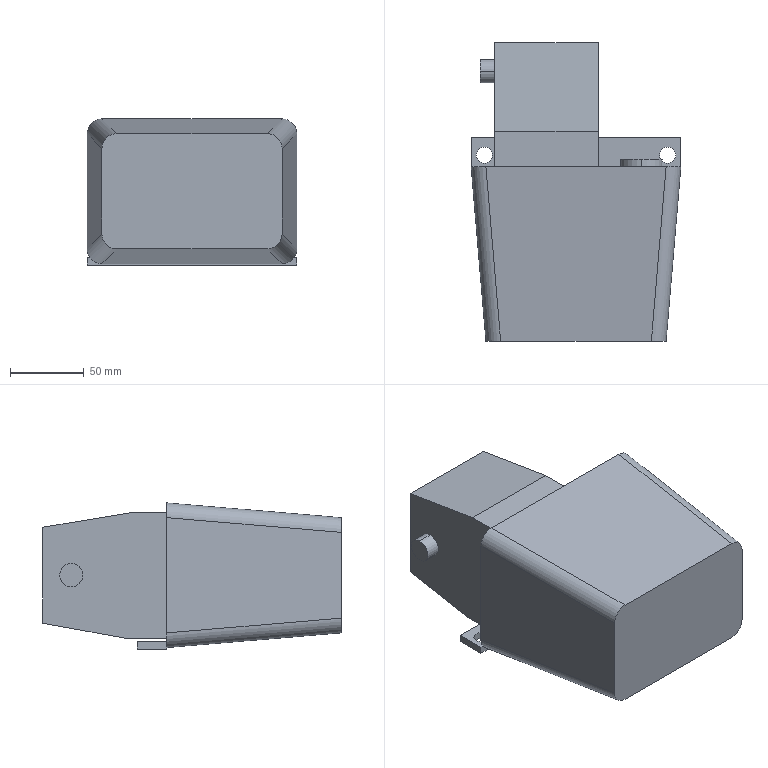Part | SolidWorks | features BaseBody 1 | 1 solid | 43 faces | box 142 x 202 x 99 mm | volume 619754 mm3 | plane 27 | cylinder 16 | commonest cylinder face diameters 11 x4 16 x4 20 x4 15.743 x2 28.298 x2
STEP:
#1=CARTESIAN_POINT('',(44.366,5.,1.458));
#2=VERTEX_POINT('',#1);
#3=CARTESIAN_POINT('',(44.366,5.,29.756));
#4=VERTEX_POINT('',#3);
#5=CARTESIAN_POINT('',(44.366,5.,15.607));
#6=DIRECTION('',(0.,-1.,0.));
#7=DIRECTION('',(0.,0.,-1.));
#8=AXIS2_PLACEMENT_3D('',#5,#6,#7);
#9=CIRCLE('',#8,14.149);
#10=EDGE_CURVE('',#2,#4,#9,.T.);
#11=ORIENTED_EDGE('',*,*,#10,.T.);
#12=CARTESIAN_POINT('',(44.366,0.,29.756));
#13=VERTEX_POINT('',#12);
#14=CARTESIAN_POINT('',(44.366,5.,29.756));
#15=DIRECTION('',(0.,-1.,0.));
#16=VECTOR('',#15,1000.);
#17=LINE('',#14,#16);
#18=EDGE_CURVE('',#4,#13,#17,.T.);
#19=ORIENTED_EDGE('',*,*,#18,.T.);
#20=CARTESIAN_POINT('',(44.366,0.,1.458));
#21=VERTEX_POINT('',#20);
#22=CARTESIAN_POINT('',(44.366,0.,15.607));
#23=DIRECTION('',(0.,-1.,0.));
#24=DIRECTION('',(0.,0.,-1.));
#25=AXIS2_PLACEMENT_3D('',#22,#23,#24);
#26=CIRCLE('',#25,14.149);
#27=EDGE_CURVE('',#21,#13,#26,.T.);
#28=ORIENTED_EDGE('',*,*,#27,.F.);
#29=CARTESIAN_POINT('',(44.366,5.,1.458));
#30=DIRECTION('',(0.,-1.,0.));
#31=VECTOR('',#30,1000.);
#32=LINE('',#29,#31);
#33=EDGE_CURVE('',#2,#21,#32,.T.);
#34=ORIENTED_EDGE('',*,*,#33,.F.);
#35=EDGE_LOOP('',(#11,#19,#28,#34));
#36=FACE_OUTER_BOUND('',#35,.T.);
#37=CARTESIAN_POINT('',(44.366,5.,15.607));
#38=DIRECTION('',(0.,-1.,0.));
#39=DIRECTION('',(0.,0.,-1.));
#40=AXIS2_PLACEMENT_3D('',#37,#38,#39);
#41=CYLINDRICAL_SURFACE('',#40,14.149);
#42=ADVANCED_FACE('',(#36),#41,.T.);
#43=CARTESIAN_POINT('',(67.5,8.,-50.));
#44=VERTEX_POINT('',#43);
#45=CARTESIAN_POINT('',(56.5,8.,-50.));
#46=VERTEX_POINT('',#45);
#47=CARTESIAN_POINT('',(62.,8.,-50.));
#48=DIRECTION('',(0.,0.,-1.));
#49=DIRECTION('',(1.,0.,0.));
#50=AXIS2_PLACEMENT_3D('',#47,#48,#49);
#51=CIRCLE('',#50,5.5);
#52=EDGE_CURVE('',#44,#46,#51,.T.);
#53=ORIENTED_EDGE('',*,*,#52,.T.);
#54=CARTESIAN_POINT('',(56.5,8.,-45.));
#55=VERTEX_POINT('',#54);
#56=CARTESIAN_POINT('',(56.5,8.,-45.));
#57=DIRECTION('',(0.,0.,1.));
#58=VECTOR('',#57,1000.);
#59=LINE('',#56,#58);
#60=EDGE_CURVE('',#46,#55,#59,.T.);
#61=ORIENTED_EDGE('',*,*,#60,.T.);
#62=CARTESIAN_POINT('',(67.5,8.,-45.));
#63=VERTEX_POINT('',#62);
#64=CARTESIAN_POINT('',(62.,8.,-45.));
#65=DIRECTION('',(0.,0.,1.));
#66=DIRECTION('',(1.,0.,0.));
#67=AXIS2_PLACEMENT_3D('',#64,#65,#66);
#68=CIRCLE('',#67,5.5);
#69=EDGE_CURVE('',#55,#63,#68,.T.);
#70=ORIENTED_EDGE('',*,*,#69,.T.);
#71=CARTESIAN_POINT('',(67.5,8.,-45.));
#72=DIRECTION('',(0.,0.,1.));
#73=VECTOR('',#72,1000.);
#74=LINE('',#71,#73);
#75=EDGE_CURVE('',#44,#63,#74,.T.);
#76=ORIENTED_EDGE('',*,*,#75,.F.);
#77=EDGE_LOOP('',(#53,#61,#70,#76));
#78=FACE_OUTER_BOUND('',#77,.T.);
#79=CARTESIAN_POINT('',(62.,8.,-45.));
#80=DIRECTION('',(0.,0.,1.));
#81=DIRECTION('',(1.,0.,0.));
#82=AXIS2_PLACEMENT_3D('',#79,#80,#81);
#83=CYLINDRICAL_SURFACE('',#82,5.5);
#84=ADVANCED_FACE('',(#78),#83,.F.);
#85=CARTESIAN_POINT('',(-56.5,8.,-50.));
#86=VERTEX_POINT('',#85);
#87=CARTESIAN_POINT('',(-67.5,8.,-50.));
#88=VERTEX_POINT('',#87);
#89=CARTESIAN_POINT('',(-62.,8.,-50.));
#90=DIRECTION('',(0.,0.,-1.));
#91=DIRECTION('',(1.,0.,0.));
#92=AXIS2_PLACEMENT_3D('',#89,#90,#91);
#93=CIRCLE('',#92,5.5);
#94=EDGE_CURVE('',#86,#88,#93,.T.);
#95=ORIENTED_EDGE('',*,*,#94,.T.);
#96=CARTESIAN_POINT('',(-67.5,8.,-45.));
#97=VERTEX_POINT('',#96);
#98=CARTESIAN_POINT('',(-67.5,8.,-45.));
#99=DIRECTION('',(0.,0.,1.));
#100=VECTOR('',#99,1000.);
#101=LINE('',#98,#100);
#102=EDGE_CURVE('',#88,#97,#101,.T.);
#103=ORIENTED_EDGE('',*,*,#102,.T.);
#104=CARTESIAN_POINT('',(-56.5,8.,-45.));
#105=VERTEX_POINT('',#104);
#106=CARTESIAN_POINT('',(-62.,8.,-45.));
#107=DIRECTION('',(0.,0.,1.));
#108=DIRECTION('',(1.,0.,0.));
#109=AXIS2_PLACEMENT_3D('',#106,#107,#108);
#110=CIRCLE('',#109,5.5);
#111=EDGE_CURVE('',#97,#105,#110,.T.);
#112=ORIENTED_EDGE('',*,*,#111,.T.);
#113=CARTESIAN_POINT('',(-56.5,8.,-45.));
#114=DIRECTION('',(0.,0.,1.));
#115=VECTOR('',#114,1000.);
#116=LINE('',#113,#115);
#117=EDGE_CURVE('',#86,#105,#116,.T.);
#118=ORIENTED_EDGE('',*,*,#117,.F.);
#119=EDGE_LOOP('',(#95,#103,#112,#118));
#120=FACE_OUTER_BOUND('',#119,.T.);
#121=CARTESIAN_POINT('',(-62.,8.,-45.));
#122=DIRECTION('',(0.,0.,1.));
#123=DIRECTION('',(1.,0.,0.));
#124=AXIS2_PLACEMENT_3D('',#121,#122,#123);
#125=CYLINDRICAL_SURFACE('',#124,5.5);
#126=ADVANCED_FACE('',(#120),#125,.F.);
#127=CARTESIAN_POINT('',(-65.,64.732,-7.871));
#128=VERTEX_POINT('',#127);
#129=CARTESIAN_POINT('',(-65.,64.732,7.871));
#130=VERTEX_POINT('',#129);
#131=CARTESIAN_POINT('',(-65.,64.732,0.));
#132=DIRECTION('',(1.,0.,0.));
#133=DIRECTION('',(0.,0.,-1.));
#134=AXIS2_PLACEMENT_3D('',#131,#132,#133);
#135=CIRCLE('',#134,7.871);
#136=EDGE_CURVE('',#128,#130,#135,.T.);
#137=ORIENTED_EDGE('',*,*,#136,.T.);
#138=CARTESIAN_POINT('',(-55.,64.732,7.871));
#139=VERTEX_POINT('',#138);
#140=CARTESIAN_POINT('',(-65.,64.732,7.871));
#141=DIRECTION('',(1.,0.,0.));
#142=VECTOR('',#141,1000.);
#143=LINE('',#140,#142);
#144=EDGE_CURVE('',#130,#139,#143,.T.);
#145=ORIENTED_EDGE('',*,*,#144,.T.);
#146=CARTESIAN_POINT('',(-55.,64.732,-7.871));
#147=VERTEX_POINT('',#146);
#148=CARTESIAN_POINT('',(-55.,64.732,0.));
#149=DIRECTION('',(-1.,0.,0.));
#150=DIRECTION('',(0.,0.,-1.));
#151=AXIS2_PLACEMENT_3D('',#148,#149,#150);
#152=CIRCLE('',#151,7.871);
#153=EDGE_CURVE('',#139,#147,#152,.T.);
#154=ORIENTED_EDGE('',*,*,#153,.T.);
#155=CARTESIAN_POINT('',(-65.,64.732,-7.871));
#156=DIRECTION('',(1.,0.,0.));
#157=VECTOR('',#156,1000.);
#158=LINE('',#155,#157);
#159=EDGE_CURVE('',#128,#147,#158,.T.);
#160=ORIENTED_EDGE('',*,*,#159,.F.);
#161=EDGE_LOOP('',(#137,#145,#154,#160));
#162=FACE_OUTER_BOUND('',#161,.T.);
#163=CARTESIAN_POINT('',(-65.,64.732,0.));
#164=DIRECTION('',(1.,0.,0.));
#165=DIRECTION('',(0.,0.,-1.));
#166=AXIS2_PLACEMENT_3D('',#163,#164,#165);
#167=CYLINDRICAL_SURFACE('',#166,7.871);
#168=ADVANCED_FACE('',(#162),#167,.T.);
#169=ORIENTED_EDGE('',*,*,#136,.F.);
#170=CARTESIAN_POINT('',(-65.,64.732,0.));
#171=DIRECTION('',(1.,0.,0.));
#172=DIRECTION('',(0.,0.,-1.));
#173=AXIS2_PLACEMENT_3D('',#170,#171,#172);
#174=CIRCLE('',#173,7.871);
#175=EDGE_CURVE('',#130,#128,#174,.T.);
#176=ORIENTED_EDGE('',*,*,#175,.F.);
#177=EDGE_LOOP('',(#169,#176));
#178=FACE_OUTER_BOUND('',#177,.T.);
#179=CARTESIAN_POINT('',(-65.,64.732,0.));
#180=DIRECTION('',(-1.,0.,0.));
#181=DIRECTION('',(0.,0.,1.));
#182=AXIS2_PLACEMENT_3D('',#179,#180,#181);
#183=PLANE('',#182);
#184=ADVANCED_FACE('',(#178),#183,.T.);
#185=ORIENTED_EDGE('',*,*,#10,.F.);
#186=CARTESIAN_POINT('',(44.366,5.,15.607));
#187=DIRECTION('',(0.,-1.,0.));
#188=DIRECTION('',(0.,0.,-1.));
#189=AXIS2_PLACEMENT_3D('',#186,#187,#188);
#190=CIRCLE('',#189,14.149);
#191=EDGE_CURVE('',#4,#2,#190,.T.);
#192=ORIENTED_EDGE('',*,*,#191,.F.);
#193=EDGE_LOOP('',(#185,#192));
#194=FACE_OUTER_BOUND('',#193,.T.);
#195=CARTESIAN_POINT('',(44.366,5.,15.607));
#196=DIRECTION('',(0.,1.,0.));
#197=DIRECTION('',(0.,0.,1.));
#198=AXIS2_PLACEMENT_3D('',#195,#196,#197);
#199=PLANE('',#198);
#200=ADVANCED_FACE('',(#194),#199,.T.);
#201=ORIENTED_EDGE('',*,*,#144,.F.);
#202=ORIENTED_EDGE('',*,*,#175,.T.);
#203=ORIENTED_EDGE('',*,*,#159,.T.);
#204=CARTESIAN_POINT('',(-55.,64.732,0.));
#205=DIRECTION('',(-1.,0.,0.));
#206=DIRECTION('',(0.,0.,-1.));
#207=AXIS2_PLACEMENT_3D('',#204,#205,#206);
#208=CIRCLE('',#207,7.871);
#209=EDGE_CURVE('',#147,#139,#208,.T.);
#210=ORIENTED_EDGE('',*,*,#209,.T.);
#211=EDGE_LOOP('',(#201,#202,#203,#210));
#212=FACE_OUTER_BOUND('',#211,.T.);
#213=CARTESIAN_POINT('',(-65.,64.732,0.));
#214=DIRECTION('',(1.,0.,0.));
#215=DIRECTION('',(0.,0.,-1.));
#216=AXIS2_PLACEMENT_3D('',#213,#214,#215);
#217=CYLINDRICAL_SURFACE('',#216,7.871);
#218=ADVANCED_FACE('',(#212),#217,.T.);
#219=CARTESIAN_POINT('',(-55.,29.,-42.5));
#220=VERTEX_POINT('',#219);
#221=CARTESIAN_POINT('',(-55.,84.,-32.5));
#222=VERTEX_POINT('',#221);
#223=CARTESIAN_POINT('',(-55.,29.,-42.5));
#224=DIRECTION('',(0.,0.9839,0.1789));
#225=VECTOR('',#224,1000.);
#226=LINE('',#223,#225);
#227=EDGE_CURVE('',#220,#222,#226,.T.);
#228=ORIENTED_EDGE('',*,*,#227,.T.);
#229=CARTESIAN_POINT('',(15.,84.,-32.5));
#230=VERTEX_POINT('',#229);
#231=CARTESIAN_POINT('',(0.,84.,-32.5));
#232=DIRECTION('',(-1.,0.,0.));
#233=VECTOR('',#232,1000.);
#234=LINE('',#231,#233);
#235=EDGE_CURVE('',#230,#222,#234,.T.);
#236=ORIENTED_EDGE('',*,*,#235,.F.);
#237=CARTESIAN_POINT('',(15.,29.,-42.5));
#238=VERTEX_POINT('',#237);
#239=CARTESIAN_POINT('',(15.,84.,-32.5));
#240=DIRECTION('',(0.,-0.9839,-0.1789));
#241=VECTOR('',#240,1000.);
#242=LINE('',#239,#241);
#243=EDGE_CURVE('',#230,#238,#242,.T.);
#244=ORIENTED_EDGE('',*,*,#243,.T.);
#245=CARTESIAN_POINT('',(-55.,29.,-42.5));
#246=DIRECTION('',(-1.,0.,0.));
#247=VECTOR('',#246,1000.);
#248=LINE('',#245,#247);
#249=EDGE_CURVE('',#238,#220,#248,.T.);
#250=ORIENTED_EDGE('',*,*,#249,.T.);
#251=EDGE_LOOP('',(#228,#236,#244,#250));
#252=FACE_OUTER_BOUND('',#251,.T.);
#253=CARTESIAN_POINT('',(71.,29.,-42.5));
#254=DIRECTION('',(0.,-0.1789,0.9839));
#255=DIRECTION('',(0.,-0.9839,-0.1789));
#256=AXIS2_PLACEMENT_3D('',#253,#254,#255);
#257=PLANE('',#256);
#258=ADVANCED_FACE('',(#252),#257,.F.);
#259=ORIENTED_EDGE('',*,*,#235,.T.);
#260=CARTESIAN_POINT('',(-55.,84.,32.5));
#261=VERTEX_POINT('',#260);
#262=CARTESIAN_POINT('',(-55.,84.,-42.5));
#263=DIRECTION('',(0.,0.,1.));
#264=VECTOR('',#263,1000.);
#265=LINE('',#262,#264);
#266=EDGE_CURVE('',#222,#261,#265,.T.);
#267=ORIENTED_EDGE('',*,*,#266,.T.);
#268=CARTESIAN_POINT('',(15.,84.,32.5));
#269=VERTEX_POINT('',#268);
#270=CARTESIAN_POINT('',(71.,84.,32.5));
#271=DIRECTION('',(1.,0.,0.));
#272=VECTOR('',#271,1000.);
#273=LINE('',#270,#272);
#274=EDGE_CURVE('',#261,#269,#273,.T.);
#275=ORIENTED_EDGE('',*,*,#274,.T.);
#276=CARTESIAN_POINT('',(15.,84.,-42.5));
#277=DIRECTION('',(0.,0.,-1.));
#278=VECTOR('',#277,1000.);
#279=LINE('',#276,#278);
#280=EDGE_CURVE('',#269,#230,#279,.T.);
#281=ORIENTED_EDGE('',*,*,#280,.T.);
#282=EDGE_LOOP('',(#259,#267,#275,#281));
#283=FACE_OUTER_BOUND('',#282,.T.);
#284=CARTESIAN_POINT('',(0.,84.,0.));
#285=DIRECTION('',(0.,1.,0.));
#286=DIRECTION('',(0.,0.,1.));
#287=AXIS2_PLACEMENT_3D('',#284,#285,#286);
#288=PLANE('',#287);
#289=ADVANCED_FACE('',(#283),#288,.T.);
#290=CARTESIAN_POINT('',(-55.,24.,42.5));
#291=VERTEX_POINT('',#290);
#292=CARTESIAN_POINT('',(-55.,84.,32.5));
#293=DIRECTION('',(0.,-0.9864,0.1644));
#294=VECTOR('',#293,1000.);
#295=LINE('',#292,#294);
#296=EDGE_CURVE('',#261,#291,#295,.T.);
#297=ORIENTED_EDGE('',*,*,#296,.T.);
#298=CARTESIAN_POINT('',(15.,24.,42.5));
#299=VERTEX_POINT('',#298);
#300=CARTESIAN_POINT('',(-55.,24.,42.5));
#301=DIRECTION('',(1.,0.,0.));
#302=VECTOR('',#301,1000.);
#303=LINE('',#300,#302);
#304=EDGE_CURVE('',#291,#299,#303,.T.);
#305=ORIENTED_EDGE('',*,*,#304,.T.);
#306=CARTESIAN_POINT('',(15.,24.,42.5));
#307=DIRECTION('',(0.,0.9864,-0.1644));
#308=VECTOR('',#307,1000.);
#309=LINE('',#306,#308);
#310=EDGE_CURVE('',#299,#269,#309,.T.);
#311=ORIENTED_EDGE('',*,*,#310,.T.);
#312=ORIENTED_EDGE('',*,*,#274,.F.);
#313=EDGE_LOOP('',(#297,#305,#311,#312));
#314=FACE_OUTER_BOUND('',#313,.T.);
#315=CARTESIAN_POINT('',(71.,84.,32.5));
#316=DIRECTION('',(0.,-0.1644,-0.9864));
#317=DIRECTION('',(0.,0.9864,-0.1644));
#318=AXIS2_PLACEMENT_3D('',#315,#316,#317);
#319=PLANE('',#318);
#320=ADVANCED_FACE('',(#314),#319,.F.);
#321=ORIENTED_EDGE('',*,*,#102,.F.);
#322=CARTESIAN_POINT('',(-62.,8.,-50.));
#323=DIRECTION('',(0.,0.,-1.));
#324=DIRECTION('',(1.,0.,0.));
#325=AXIS2_PLACEMENT_3D('',#322,#323,#324);
#326=CIRCLE('',#325,5.5);
#327=EDGE_CURVE('',#88,#86,#326,.T.);
#328=ORIENTED_EDGE('',*,*,#327,.T.);
#329=ORIENTED_EDGE('',*,*,#117,.T.);
#330=CARTESIAN_POINT('',(-62.,8.,-45.));
#331=DIRECTION('',(0.,0.,1.));
#332=DIRECTION('',(1.,0.,0.));
#333=AXIS2_PLACEMENT_3D('',#330,#331,#332);
#334=CIRCLE('',#333,5.5);
#335=EDGE_CURVE('',#105,#97,#334,.T.);
#336=ORIENTED_EDGE('',*,*,#335,.T.);
#337=EDGE_LOOP('',(#321,#328,#329,#336));
#338=FACE_OUTER_BOUND('',#337,.T.);
#339=CARTESIAN_POINT('',(-62.,8.,-45.));
#340=DIRECTION('',(0.,0.,1.));
#341=DIRECTION('',(1.,0.,0.));
#342=AXIS2_PLACEMENT_3D('',#339,#340,#341);
#343=CYLINDRICAL_SURFACE('',#342,5.5);
#344=ADVANCED_FACE('',(#338),#343,.F.);
#345=ORIENTED_EDGE('',*,*,#60,.F.);
#346=CARTESIAN_POINT('',(62.,8.,-50.));
#347=DIRECTION('',(0.,0.,-1.));
#348=DIRECTION('',(1.,0.,0.));
#349=AXIS2_PLACEMENT_3D('',#346,#347,#348);
#350=CIRCLE('',#349,5.5);
#351=EDGE_CURVE('',#46,#44,#350,.T.);
#352=ORIENTED_EDGE('',*,*,#351,.T.);
#353=ORIENTED_EDGE('',*,*,#75,.T.);
#354=CARTESIAN_POINT('',(62.,8.,-45.));
#355=DIRECTION('',(0.,0.,1.));
#356=DIRECTION('',(1.,0.,0.));
#357=AXIS2_PLACEMENT_3D('',#354,#355,#356);
#358=CIRCLE('',#357,5.5);
#359=EDGE_CURVE('',#63,#55,#358,.T.);
#360=ORIENTED_EDGE('',*,*,#359,.T.);
#361=EDGE_LOOP('',(#345,#352,#353,#360));
#362=FACE_OUTER_BOUND('',#361,.T.);
#363=CARTESIAN_POINT('',(62.,8.,-45.));
#364=DIRECTION('',(0.,0.,1.));
#365=DIRECTION('',(1.,0.,0.));
#366=AXIS2_PLACEMENT_3D('',#363,#364,#365);
#367=CYLINDRICAL_SURFACE('',#366,5.5);
#368=ADVANCED_FACE('',(#362),#367,.F.);
#369=CARTESIAN_POINT('',(-71.,20.,-50.));
#370=VERTEX_POINT('',#369);
#371=CARTESIAN_POINT('',(-71.,20.,-45.));
#372=VERTEX_POINT('',#371);
#373=CARTESIAN_POINT('',(-71.,20.,-45.));
#374=DIRECTION('',(0.,0.,1.));
#375=VECTOR('',#374,1000.);
#376=LINE('',#373,#375);
#377=EDGE_CURVE('',#370,#372,#376,.T.);
#378=ORIENTED_EDGE('',*,*,#377,.T.);
#379=CARTESIAN_POINT('',(71.,20.,-45.));
#380=VERTEX_POINT('',#379);
#381=CARTESIAN_POINT('',(71.,20.,-45.));
#382=DIRECTION('',(1.,0.,0.));
#383=VECTOR('',#382,1000.);
#384=LINE('',#381,#383);
#385=EDGE_CURVE('',#372,#380,#384,.T.);
#386=ORIENTED_EDGE('',*,*,#385,.T.);
#387=CARTESIAN_POINT('',(71.,20.,-50.));
#388=VERTEX_POINT('',#387);
#389=CARTESIAN_POINT('',(71.,20.,-45.));
#390=DIRECTION('',(0.,0.,-1.));
#391=VECTOR('',#390,1000.);
#392=LINE('',#389,#391);
#393=EDGE_CURVE('',#380,#388,#392,.T.);
#394=ORIENTED_EDGE('',*,*,#393,.T.);
#395=CARTESIAN_POINT('',(71.,20.,-50.));
#396=DIRECTION('',(-1.,0.,0.));
#397=VECTOR('',#396,1000.);
#398=LINE('',#395,#397);
#399=EDGE_CURVE('',#388,#370,#398,.T.);
#400=ORIENTED_EDGE('',*,*,#399,.T.);
#401=EDGE_LOOP('',(#378,#386,#394,#400));
#402=FACE_OUTER_BOUND('',#401,.T.);
#403=CARTESIAN_POINT('',(0.,20.,0.));
#404=DIRECTION('',(0.,1.,0.));
#405=DIRECTION('',(0.,0.,1.));
#406=AXIS2_PLACEMENT_3D('',#403,#404,#405);
#407=PLANE('',#406);
#408=ADVANCED_FACE('',(#402),#407,.T.);
#409=ORIENTED_EDGE('',*,*,#18,.F.);
#410=ORIENTED_EDGE('',*,*,#191,.T.);
#411=ORIENTED_EDGE('',*,*,#33,.T.);
#412=CARTESIAN_POINT('',(44.366,0.,15.607));
#413=DIRECTION('',(0.,-1.,0.));
#414=DIRECTION('',(0.,0.,-1.));
#415=AXIS2_PLACEMENT_3D('',#412,#413,#414);
#416=CIRCLE('',#415,14.149);
#417=EDGE_CURVE('',#13,#21,#416,.T.);
#418=ORIENTED_EDGE('',*,*,#417,.F.);
#419=EDGE_LOOP('',(#409,#410,#411,#418));
#420=FACE_OUTER_BOUND('',#419,.T.);
#421=CARTESIAN_POINT('',(44.366,5.,15.607));
#422=DIRECTION('',(0.,-1.,0.));
#423=DIRECTION('',(0.,0.,-1.));
#424=AXIS2_PLACEMENT_3D('',#421,#422,#423);
#425=CYLINDRICAL_SURFACE('',#424,14.149);
#426=ADVANCED_FACE('',(#420),#425,.T.);
#427=ORIENTED_EDGE('',*,*,#296,.F.);
#428=ORIENTED_EDGE('',*,*,#266,.F.);
#429=ORIENTED_EDGE('',*,*,#227,.F.);
#430=CARTESIAN_POINT('',(-55.,0.,-42.5));
#431=VERTEX_POINT('',#430);
#432=CARTESIAN_POINT('',(-55.,84.,-42.5));
#433=DIRECTION('',(0.,-1.,0.));
#434=VECTOR('',#433,1000.);
#435=LINE('',#432,#434);
#436=EDGE_CURVE('',#220,#431,#435,.T.);
#437=ORIENTED_EDGE('',*,*,#436,.T.);
#438=CARTESIAN_POINT('',(-55.,0.,42.5));
#439=VERTEX_POINT('',#438);
#440=CARTESIAN_POINT('',(-55.,0.,0.));
#441=DIRECTION('',(0.,0.,-1.));
#442=VECTOR('',#441,1000.);
#443=LINE('',#440,#442);
#444=EDGE_CURVE('',#439,#431,#443,.T.);
#445=ORIENTED_EDGE('',*,*,#444,.F.);
#446=CARTESIAN_POINT('',(-55.,84.,42.5));
#447=DIRECTION('',(0.,1.,0.));
#448=VECTOR('',#447,1000.);
#449=LINE('',#446,#448);
#450=EDGE_CURVE('',#439,#291,#449,.T.);
#451=ORIENTED_EDGE('',*,*,#450,.T.);
#452=EDGE_LOOP('',(#427,#428,#429,#437,#445,#451));
#453=FACE_OUTER_BOUND('',#452,.T.);
#454=ORIENTED_EDGE('',*,*,#209,.F.);
#455=ORIENTED_EDGE('',*,*,#153,.F.);
#456=EDGE_LOOP('',(#454,#455));
#457=FACE_BOUND('',#456,.T.);
#458=CARTESIAN_POINT('',(-55.,84.,-42.5));
#459=DIRECTION('',(1.,0.,0.));
#460=DIRECTION('',(0.,0.,-1.));
#461=AXIS2_PLACEMENT_3D('',#458,#459,#460);
#462=PLANE('',#461);
#463=ADVANCED_FACE('',(#453,#457),#462,.F.);
#464=ORIENTED_EDGE('',*,*,#249,.F.);
#465=CARTESIAN_POINT('',(15.,0.,-42.5));
#466=VERTEX_POINT('',#465);
#467=CARTESIAN_POINT('',(15.,84.,-42.5));
#468=DIRECTION('',(0.,-1.,0.));
#469=VECTOR('',#468,1000.);
#470=LINE('',#467,#469);
#471=EDGE_CURVE('',#238,#466,#470,.T.);
#472=ORIENTED_EDGE('',*,*,#471,.T.);
#473=CARTESIAN_POINT('',(0.,0.,-42.5));
#474=DIRECTION('',(1.,0.,0.));
#475=VECTOR('',#474,1000.);
#476=LINE('',#473,#475);
#477=EDGE_CURVE('',#431,#466,#476,.T.);
#478=ORIENTED_EDGE('',*,*,#477,.F.);
#479=ORIENTED_EDGE('',*,*,#436,.F.);
#480=EDGE_LOOP('',(#464,#472,#478,#479));
#481=FACE_OUTER_BOUND('',#480,.T.);
#482=CARTESIAN_POINT('',(-55.,84.,-42.5));
#483=DIRECTION('',(0.,0.,1.));
#484=DIRECTION('',(1.,0.,0.));
#485=AXIS2_PLACEMENT_3D('',#482,#483,#484);
#486=PLANE('',#485);
#487=ADVANCED_FACE('',(#481),#486,.F.);
#488=ORIENTED_EDGE('',*,*,#310,.F.);
#489=CARTESIAN_POINT('',(15.,0.,42.5));
#490=VERTEX_POINT('',#489);
#491=CARTESIAN_POINT('',(15.,84.,42.5));
#492=DIRECTION('',(0.,-1.,0.));
#493=VECTOR('',#492,1000.);
#494=LINE('',#491,#493);
#495=EDGE_CURVE('',#299,#490,#494,.T.);
#496=ORIENTED_EDGE('',*,*,#495,.T.);
#497=CARTESIAN_POINT('',(15.,0.,0.));
#498=DIRECTION('',(0.,0.,1.));
#499=VECTOR('',#498,1000.);
#500=LINE('',#497,#499);
#501=EDGE_CURVE('',#466,#490,#500,.T.);
#502=ORIENTED_EDGE('',*,*,#501,.F.);
#503=ORIENTED_EDGE('',*,*,#471,.F.);
#504=ORIENTED_EDGE('',*,*,#243,.F.);
#505=ORIENTED_EDGE('',*,*,#280,.F.);
#506=EDGE_LOOP('',(#488,#496,#502,#503,#504,#505));
#507=FACE_OUTER_BOUND('',#506,.T.);
#508=CARTESIAN_POINT('',(15.,84.,-42.5));
#509=DIRECTION('',(-1.,0.,0.));
#510=DIRECTION('',(0.,0.,1.));
#511=AXIS2_PLACEMENT_3D('',#508,#509,#510);
#512=PLANE('',#511);
#513=ADVANCED_FACE('',(#507),#512,.F.);
#514=ORIENTED_EDGE('',*,*,#304,.F.);
#515=ORIENTED_EDGE('',*,*,#450,.F.);
#516=CARTESIAN_POINT('',(0.,0.,42.5));
#517=DIRECTION('',(-1.,0.,0.));
#518=VECTOR('',#517,1000.);
#519=LINE('',#516,#518);
#520=EDGE_CURVE('',#490,#439,#519,.T.);
#521=ORIENTED_EDGE('',*,*,#520,.F.);
#522=ORIENTED_EDGE('',*,*,#495,.F.);
#523=EDGE_LOOP('',(#514,#515,#521,#522));
#524=FACE_OUTER_BOUND('',#523,.T.);
#525=CARTESIAN_POINT('',(-55.,84.,42.5));
#526=DIRECTION('',(0.,0.,-1.));
#527=DIRECTION('',(-1.,0.,0.));
#528=AXIS2_PLACEMENT_3D('',#525,#526,#527);
#529=PLANE('',#528);
#530=ADVANCED_FACE('',(#524),#529,.F.);
#531=CARTESIAN_POINT('',(71.,0.,-50.));
#532=VERTEX_POINT('',#531);
#533=CARTESIAN_POINT('',(71.,20.,-50.));
#534=DIRECTION('',(0.,1.,0.));
#535=VECTOR('',#534,1000.);
#536=LINE('',#533,#535);
#537=EDGE_CURVE('',#532,#388,#536,.T.);
#538=ORIENTED_EDGE('',*,*,#537,.T.);
#539=ORIENTED_EDGE('',*,*,#393,.F.);
#540=CARTESIAN_POINT('',(71.,0.,-45.));
#541=VERTEX_POINT('',#540);
#542=CARTESIAN_POINT('',(71.,20.,-45.));
#543=DIRECTION('',(0.,-1.,0.));
#544=VECTOR('',#543,1000.);
#545=LINE('',#542,#544);
#546=EDGE_CURVE('',#380,#541,#545,.T.);
#547=ORIENTED_EDGE('',*,*,#546,.T.);
#548=CARTESIAN_POINT('',(71.,0.,0.));
#549=DIRECTION('',(0.,0.,-1.));
#550=VECTOR('',#549,1000.);
#551=LINE('',#548,#550);
#552=EDGE_CURVE('',#541,#532,#551,.T.);
#553=ORIENTED_EDGE('',*,*,#552,.T.);
#554=EDGE_LOOP('',(#538,#539,#547,#553));
#555=FACE_OUTER_BOUND('',#554,.T.);
#556=CARTESIAN_POINT('',(71.,20.,-45.));
#557=DIRECTION('',(-1.,0.,0.));
#558=DIRECTION('',(0.,0.,1.));
#559=AXIS2_PLACEMENT_3D('',#556,#557,#558);
#560=PLANE('',#559);
#561=ADVANCED_FACE('',(#555),#560,.F.);
#562=CARTESIAN_POINT('',(-71.,0.,-50.));
#563=VERTEX_POINT('',#562);
#564=CARTESIAN_POINT('',(-71.,20.,-50.));
#565=DIRECTION('',(0.,1.,0.));
#566=VECTOR('',#565,1000.);
#567=LINE('',#564,#566);
#568=EDGE_CURVE('',#563,#370,#567,.T.);
#569=ORIENTED_EDGE('',*,*,#568,.T.);
#570=ORIENTED_EDGE('',*,*,#399,.F.);
#571=ORIENTED_EDGE('',*,*,#537,.F.);
#572=CARTESIAN_POINT('',(0.,0.,-50.));
#573=DIRECTION('',(-1.,0.,0.));
#574=VECTOR('',#573,1000.);
#575=LINE('',#572,#574);
#576=EDGE_CURVE('',#532,#563,#575,.T.);
#577=ORIENTED_EDGE('',*,*,#576,.T.);
#578=EDGE_LOOP('',(#569,#570,#571,#577));
#579=FACE_OUTER_BOUND('',#578,.T.);
#580=ORIENTED_EDGE('',*,*,#52,.F.);
#581=ORIENTED_EDGE('',*,*,#351,.F.);
#582=EDGE_LOOP('',(#580,#581));
#583=FACE_BOUND('',#582,.T.);
#584=ORIENTED_EDGE('',*,*,#94,.F.);
#585=ORIENTED_EDGE('',*,*,#327,.F.);
#586=EDGE_LOOP('',(#584,#585));
#587=FACE_BOUND('',#586,.T.);
#588=CARTESIAN_POINT('',(71.,20.,-50.));
#589=DIRECTION('',(0.,0.,1.));
#590=DIRECTION('',(1.,0.,0.));
#591=AXIS2_PLACEMENT_3D('',#588,#589,#590);
#592=PLANE('',#591);
#593=ADVANCED_FACE('',(#579,#583,#587),#592,.F.);
#594=CARTESIAN_POINT('',(-71.,0.,-45.));
#595=VERTEX_POINT('',#594);
#596=CARTESIAN_POINT('',(-71.,20.,-45.));
#597=DIRECTION('',(0.,1.,0.));
#598=VECTOR('',#597,1000.);
#599=LINE('',#596,#598);
#600=EDGE_CURVE('',#595,#372,#599,.T.);
#601=ORIENTED_EDGE('',*,*,#600,.T.);
#602=ORIENTED_EDGE('',*,*,#377,.F.);
#603=ORIENTED_EDGE('',*,*,#568,.F.);
#604=CARTESIAN_POINT('',(-71.,0.,0.));
#605=DIRECTION('',(0.,0.,1.));
#606=VECTOR('',#605,1000.);
#607=LINE('',#604,#606);
#608=EDGE_CURVE('',#563,#595,#607,.T.);
#609=ORIENTED_EDGE('',*,*,#608,.T.);
#610=EDGE_LOOP('',(#601,#602,#603,#609));
#611=FACE_OUTER_BOUND('',#610,.T.);
#612=CARTESIAN_POINT('',(-71.,20.,-45.));
#613=DIRECTION('',(1.,0.,0.));
#614=DIRECTION('',(0.,0.,-1.));
#615=AXIS2_PLACEMENT_3D('',#612,#613,#614);
#616=PLANE('',#615);
#617=ADVANCED_FACE('',(#611),#616,.F.);
#618=CARTESIAN_POINT('',(69.025,0.,-45.));
#619=VERTEX_POINT('',#618);
#620=CARTESIAN_POINT('',(-69.025,0.,-45.));
#621=VERTEX_POINT('',#620);
#622=CARTESIAN_POINT('',(0.,0.,-45.));
#623=DIRECTION('',(-1.,0.,0.));
#624=VECTOR('',#623,1000.);
#625=LINE('',#622,#624);
#626=EDGE_CURVE('',#619,#621,#625,.T.);
#627=ORIENTED_EDGE('',*,*,#626,.F.);
#628=CARTESIAN_POINT('',(0.,0.,-45.));
#629=DIRECTION('',(1.,0.,0.));
#630=VECTOR('',#629,1000.);
#631=LINE('',#628,#630);
#632=EDGE_CURVE('',#619,#541,#631,.T.);
#633=ORIENTED_EDGE('',*,*,#632,.T.);
#634=ORIENTED_EDGE('',*,*,#546,.F.);
#635=ORIENTED_EDGE('',*,*,#385,.F.);
#636=ORIENTED_EDGE('',*,*,#600,.F.);
#637=CARTESIAN_POINT('',(0.,0.,-45.));
#638=DIRECTION('',(1.,0.,0.));
#639=VECTOR('',#638,1000.);
#640=LINE('',#637,#639);
#641=EDGE_CURVE('',#595,#621,#640,.T.);
#642=ORIENTED_EDGE('',*,*,#641,.T.);
#643=EDGE_LOOP('',(#627,#633,#634,#635,#636,#642));
#644=FACE_OUTER_BOUND('',#643,.T.);
#645=ORIENTED_EDGE('',*,*,#359,.F.);
#646=ORIENTED_EDGE('',*,*,#69,.F.);
#647=EDGE_LOOP('',(#645,#646));
#648=FACE_BOUND('',#647,.T.);
#649=ORIENTED_EDGE('',*,*,#335,.F.);
#650=ORIENTED_EDGE('',*,*,#111,.F.);
#651=EDGE_LOOP('',(#649,#650));
#652=FACE_BOUND('',#651,.T.);
#653=CARTESIAN_POINT('',(71.,20.,-45.));
#654=DIRECTION('',(0.,0.,-1.));
#655=DIRECTION('',(-1.,0.,0.));
#656=AXIS2_PLACEMENT_3D('',#653,#654,#655);
#657=PLANE('',#656);
#658=ADVANCED_FACE('',(#644,#648,#652),#657,.F.);
#659=CARTESIAN_POINT('',(71.,0.,39.036));
#660=VERTEX_POINT('',#659);
#661=CARTESIAN_POINT('',(61.036,0.,49.));
#662=VERTEX_POINT('',#661);
#663=CARTESIAN_POINT('',(71.,0.,39.036));
#664=CARTESIAN_POINT('',(71.,0.,44.881));
#665=CARTESIAN_POINT('',(66.881,0.,49.));
#666=CARTESIAN_POINT('',(61.036,0.,49.));
#667=(BOUNDED_CURVE()B_SPLINE_CURVE(3,(#663,#664,#665,#666),.UNSPECIFIED.,.F.,.F.)B_SPLINE_CURVE_WITH_KNOTS((4,4),(5.501,7.065),.UNSPECIFIED.)CURVE()GEOMETRIC_REPRESENTATION_ITEM()RATIONAL_B_SPLINE_CURVE((1.,0.8064,0.8064,1.))REPRESENTATION_ITEM(''));
#668=EDGE_CURVE('',#660,#662,#667,.T.);
#669=ORIENTED_EDGE('',*,*,#668,.F.);
#670=CARTESIAN_POINT('',(71.,0.,-39.036));
#671=VERTEX_POINT('',#670);
#672=CARTESIAN_POINT('',(71.,0.,0.));
#673=DIRECTION('',(0.,0.,-1.));
#674=VECTOR('',#673,1000.);
#675=LINE('',#672,#674);
#676=EDGE_CURVE('',#660,#671,#675,.T.);
#677=ORIENTED_EDGE('',*,*,#676,.T.);
#678=CARTESIAN_POINT('',(69.025,0.,-45.));
#679=CARTESIAN_POINT('',(70.319,0.,-43.265));
#680=CARTESIAN_POINT('',(71.,0.,-41.208));
#681=CARTESIAN_POINT('',(71.,0.,-39.036));
#682=(BOUNDED_CURVE()B_SPLINE_CURVE(3,(#678,#679,#680,#681),.UNSPECIFIED.,.F.,.F.)B_SPLINE_CURVE_WITH_KNOTS((4,4),(0.1437,0.7818),.UNSPECIFIED.)CURVE()GEOMETRIC_REPRESENTATION_ITEM()RATIONAL_B_SPLINE_CURVE((1.,0.9663,0.9663,1.))REPRESENTATION_ITEM(''));
#683=EDGE_CURVE('',#619,#671,#682,.T.);
#684=ORIENTED_EDGE('',*,*,#683,.F.);
#685=ORIENTED_EDGE('',*,*,#626,.T.);
#686=CARTESIAN_POINT('',(-71.,0.,-39.036));
#687=VERTEX_POINT('',#686);
#688=CARTESIAN_POINT('',(-71.,0.,-39.036));
#689=CARTESIAN_POINT('',(-71.,0.,-41.208));
#690=CARTESIAN_POINT('',(-70.319,0.,-43.265));
#691=CARTESIAN_POINT('',(-69.025,0.,-45.));
#692=(BOUNDED_CURVE()B_SPLINE_CURVE(3,(#688,#689,#690,#691),.UNSPECIFIED.,.F.,.F.)B_SPLINE_CURVE_WITH_KNOTS((4,4),(5.501,6.14),.UNSPECIFIED.)CURVE()GEOMETRIC_REPRESENTATION_ITEM()RATIONAL_B_SPLINE_CURVE((1.,0.9663,0.9663,1.))REPRESENTATION_ITEM(''));
#693=EDGE_CURVE('',#687,#621,#692,.T.);
#694=ORIENTED_EDGE('',*,*,#693,.F.);
#695=CARTESIAN_POINT('',(-71.,0.,39.036));
#696=VERTEX_POINT('',#695);
#697=CARTESIAN_POINT('',(-71.,0.,0.));
#698=DIRECTION('',(0.,0.,1.));
#699=VECTOR('',#698,1000.);
#700=LINE('',#697,#699);
#701=EDGE_CURVE('',#687,#696,#700,.T.);
#702=ORIENTED_EDGE('',*,*,#701,.T.);
#703=CARTESIAN_POINT('',(-61.036,0.,49.));
#704=VERTEX_POINT('',#703);
#705=CARTESIAN_POINT('',(-61.036,0.,49.));
#706=CARTESIAN_POINT('',(-66.881,0.,49.));
#707=CARTESIAN_POINT('',(-71.,0.,44.881));
#708=CARTESIAN_POINT('',(-71.,0.,39.036));
#709=(BOUNDED_CURVE()B_SPLINE_CURVE(3,(#705,#706,#707,#708),.UNSPECIFIED.,.F.,.F.)B_SPLINE_CURVE_WITH_KNOTS((4,4),(5.501,7.065),.UNSPECIFIED.)CURVE()GEOMETRIC_REPRESENTATION_ITEM()RATIONAL_B_SPLINE_CURVE((1.,0.8064,0.8064,1.))REPRESENTATION_ITEM(''));
#710=EDGE_CURVE('',#704,#696,#709,.T.);
#711=ORIENTED_EDGE('',*,*,#710,.F.);
#712=CARTESIAN_POINT('',(0.,0.,49.));
#713=DIRECTION('',(1.,0.,0.));
#714=VECTOR('',#713,1000.);
#715=LINE('',#712,#714);
#716=EDGE_CURVE('',#704,#662,#715,.T.);
#717=ORIENTED_EDGE('',*,*,#716,.T.);
#718=EDGE_LOOP('',(#669,#677,#684,#685,#694,#702,#711,#717));
#719=FACE_OUTER_BOUND('',#718,.T.);
#720=ORIENTED_EDGE('',*,*,#501,.T.);
#721=ORIENTED_EDGE('',*,*,#520,.T.);
#722=ORIENTED_EDGE('',*,*,#444,.T.);
#723=ORIENTED_EDGE('',*,*,#477,.T.);
#724=EDGE_LOOP('',(#720,#721,#722,#723));
#725=FACE_BOUND('',#724,.T.);
#726=ORIENTED_EDGE('',*,*,#27,.T.);
#727=ORIENTED_EDGE('',*,*,#417,.T.);
#728=EDGE_LOOP('',(#726,#727));
#729=FACE_BOUND('',#728,.T.);
#730=CARTESIAN_POINT('',(0.,0.,0.));
#731=DIRECTION('',(0.,1.,0.));
#732=DIRECTION('',(0.,0.,1.));
#733=AXIS2_PLACEMENT_3D('',#730,#731,#732);
#734=PLANE('',#733);
#735=ADVANCED_FACE('',(#719,#725,#729),#734,.T.);
#736=ORIENTED_EDGE('',*,*,#710,.T.);
#737=CARTESIAN_POINT('',(-61.,-118.,29.036));
#738=VERTEX_POINT('',#737);
#739=CARTESIAN_POINT('',(-71.,0.,39.036));
#740=DIRECTION('',(0.08414,-0.9929,-0.08414));
#741=VECTOR('',#740,1000.);
#742=LINE('',#739,#741);
#743=EDGE_CURVE('',#696,#738,#742,.T.);
#744=ORIENTED_EDGE('',*,*,#743,.T.);
#745=CARTESIAN_POINT('',(-51.036,-118.,39.));
#746=VERTEX_POINT('',#745);
#747=CARTESIAN_POINT('',(-61.,-118.,29.036));
#748=CARTESIAN_POINT('',(-61.,-118.,34.881));
#749=CARTESIAN_POINT('',(-56.881,-118.,39.));
#750=CARTESIAN_POINT('',(-51.036,-118.,39.));
#751=(BOUNDED_CURVE()B_SPLINE_CURVE(3,(#747,#748,#749,#750),.UNSPECIFIED.,.F.,.F.)B_SPLINE_CURVE_WITH_KNOTS((4,4),(5.501,7.065),.UNSPECIFIED.)CURVE()GEOMETRIC_REPRESENTATION_ITEM()RATIONAL_B_SPLINE_CURVE((1.,0.8064,0.8064,1.))REPRESENTATION_ITEM(''));
#752=EDGE_CURVE('',#738,#746,#751,.T.);
#753=ORIENTED_EDGE('',*,*,#752,.T.);
#754=CARTESIAN_POINT('',(-51.036,-118.,39.));
#755=DIRECTION('',(-0.08414,0.9929,0.08414));
#756=VECTOR('',#755,1000.);
#757=LINE('',#754,#756);
#758=EDGE_CURVE('',#746,#704,#757,.T.);
#759=ORIENTED_EDGE('',*,*,#758,.T.);
#760=EDGE_LOOP('',(#736,#744,#753,#759));
#761=FACE_OUTER_BOUND('',#760,.T.);
#762=CARTESIAN_POINT('',(-60.257,-8.349,38.257));
#763=DIRECTION('',(-0.08414,0.9929,0.08414));
#764=DIRECTION('',(0.,-0.08444,0.9964));
#765=AXIS2_PLACEMENT_3D('',#762,#763,#764);
#766=CYLINDRICAL_SURFACE('',#765,10.);
#767=ADVANCED_FACE('',(#761),#766,.T.);
#768=CARTESIAN_POINT('',(51.036,-118.,39.));
#769=VERTEX_POINT('',#768);
#770=CARTESIAN_POINT('',(60.257,-9.193,48.221));
#771=DIRECTION('',(-0.08414,-0.9929,-0.08414));
#772=VECTOR('',#771,1000.);
#773=LINE('',#770,#772);
#774=EDGE_CURVE('',#662,#769,#773,.T.);
#775=ORIENTED_EDGE('',*,*,#774,.F.);
#776=ORIENTED_EDGE('',*,*,#716,.F.);
#777=ORIENTED_EDGE('',*,*,#758,.F.);
#778=CARTESIAN_POINT('',(0.,-118.,39.));
#779=DIRECTION('',(1.,0.,0.));
#780=VECTOR('',#779,1000.);
#781=LINE('',#778,#780);
#782=EDGE_CURVE('',#746,#769,#781,.T.);
#783=ORIENTED_EDGE('',*,*,#782,.T.);
#784=EDGE_LOOP('',(#775,#776,#777,#783));
#785=FACE_OUTER_BOUND('',#784,.T.);
#786=CARTESIAN_POINT('',(0.,-4.123,48.651));
#787=DIRECTION('',(0.,0.08444,-0.9964));
#788=DIRECTION('',(0.,0.9964,0.08444));
#789=AXIS2_PLACEMENT_3D('',#786,#787,#788);
#790=PLANE('',#789);
#791=ADVANCED_FACE('',(#785),#790,.F.);
#792=ORIENTED_EDGE('',*,*,#668,.T.);
#793=ORIENTED_EDGE('',*,*,#774,.T.);
#794=CARTESIAN_POINT('',(61.,-118.,29.036));
#795=VERTEX_POINT('',#794);
#796=CARTESIAN_POINT('',(51.036,-118.,39.));
#797=CARTESIAN_POINT('',(56.881,-118.,39.));
#798=CARTESIAN_POINT('',(61.,-118.,34.881));
#799=CARTESIAN_POINT('',(61.,-118.,29.036));
#800=(BOUNDED_CURVE()B_SPLINE_CURVE(3,(#796,#797,#798,#799),.UNSPECIFIED.,.F.,.F.)B_SPLINE_CURVE_WITH_KNOTS((4,4),(5.501,7.065),.UNSPECIFIED.)CURVE()GEOMETRIC_REPRESENTATION_ITEM()RATIONAL_B_SPLINE_CURVE((1.,0.8064,0.8064,1.))REPRESENTATION_ITEM(''));
#801=EDGE_CURVE('',#769,#795,#800,.T.);
#802=ORIENTED_EDGE('',*,*,#801,.T.);
#803=CARTESIAN_POINT('',(61.,-118.,29.036));
#804=DIRECTION('',(0.08414,0.9929,0.08414));
#805=VECTOR('',#804,1000.);
#806=LINE('',#803,#805);
#807=EDGE_CURVE('',#795,#660,#806,.T.);
#808=ORIENTED_EDGE('',*,*,#807,.T.);
#809=EDGE_LOOP('',(#792,#793,#802,#808));
#810=FACE_OUTER_BOUND('',#809,.T.);
#811=CARTESIAN_POINT('',(60.257,-8.349,38.257));
#812=DIRECTION('',(0.08414,0.9929,0.08414));
#813=DIRECTION('',(0.,-0.08444,0.9964));
#814=AXIS2_PLACEMENT_3D('',#811,#812,#813);
#815=CYLINDRICAL_SURFACE('',#814,10.);
#816=ADVANCED_FACE('',(#810),#815,.T.);
#817=CARTESIAN_POINT('',(61.,-118.,-29.036));
#818=VERTEX_POINT('',#817);
#819=CARTESIAN_POINT('',(70.221,-9.193,-38.257));
#820=DIRECTION('',(-0.08414,-0.9929,0.08414));
#821=VECTOR('',#820,1000.);
#822=LINE('',#819,#821);
#823=EDGE_CURVE('',#671,#818,#822,.T.);
#824=ORIENTED_EDGE('',*,*,#823,.F.);
#825=ORIENTED_EDGE('',*,*,#676,.F.);
#826=ORIENTED_EDGE('',*,*,#807,.F.);
#827=CARTESIAN_POINT('',(61.,-118.,0.));
#828=DIRECTION('',(0.,0.,-1.));
#829=VECTOR('',#828,1000.);
#830=LINE('',#827,#829);
#831=EDGE_CURVE('',#795,#818,#830,.T.);
#832=ORIENTED_EDGE('',*,*,#831,.T.);
#833=EDGE_LOOP('',(#824,#825,#826,#832));
#834=FACE_OUTER_BOUND('',#833,.T.);
#835=CARTESIAN_POINT('',(70.494,-5.974,0.));
#836=DIRECTION('',(-0.9964,0.08444,0.));
#837=DIRECTION('',(-0.08444,-0.9964,0.));
#838=AXIS2_PLACEMENT_3D('',#835,#836,#837);
#839=PLANE('',#838);
#840=ADVANCED_FACE('',(#834),#839,.F.);
#841=CARTESIAN_POINT('',(-61.,-118.,-29.036));
#842=VERTEX_POINT('',#841);
#843=CARTESIAN_POINT('',(-70.221,-9.193,-38.257));
#844=DIRECTION('',(-0.08414,0.9929,-0.08414));
#845=VECTOR('',#844,1000.);
#846=LINE('',#843,#845);
#847=EDGE_CURVE('',#842,#687,#846,.T.);
#848=ORIENTED_EDGE('',*,*,#847,.F.);
#849=CARTESIAN_POINT('',(-61.,-118.,0.));
#850=DIRECTION('',(0.,0.,1.));
#851=VECTOR('',#850,1000.);
#852=LINE('',#849,#851);
#853=EDGE_CURVE('',#842,#738,#852,.T.);
#854=ORIENTED_EDGE('',*,*,#853,.T.);
#855=ORIENTED_EDGE('',*,*,#743,.F.);
#856=ORIENTED_EDGE('',*,*,#701,.F.);
#857=EDGE_LOOP('',(#848,#854,#855,#856));
#858=FACE_OUTER_BOUND('',#857,.T.);
#859=CARTESIAN_POINT('',(-70.494,-5.974,0.));
#860=DIRECTION('',(0.9964,0.08444,0.));
#861=DIRECTION('',(-0.08444,0.9964,0.));
#862=AXIS2_PLACEMENT_3D('',#859,#860,#861);
#863=PLANE('',#862);
#864=ADVANCED_FACE('',(#858),#863,.F.);
#865=ORIENTED_EDGE('',*,*,#683,.T.);
#866=ORIENTED_EDGE('',*,*,#823,.T.);
#867=CARTESIAN_POINT('',(51.036,-118.,-39.));
#868=VERTEX_POINT('',#867);
#869=CARTESIAN_POINT('',(61.,-118.,-29.036));
#870=CARTESIAN_POINT('',(61.,-118.,-34.881));
#871=CARTESIAN_POINT('',(56.881,-118.,-39.));
#872=CARTESIAN_POINT('',(51.036,-118.,-39.));
#873=(BOUNDED_CURVE()B_SPLINE_CURVE(3,(#869,#870,#871,#872),.UNSPECIFIED.,.F.,.F.)B_SPLINE_CURVE_WITH_KNOTS((4,4),(5.501,7.065),.UNSPECIFIED.)CURVE()GEOMETRIC_REPRESENTATION_ITEM()RATIONAL_B_SPLINE_CURVE((1.,0.8064,0.8064,1.))REPRESENTATION_ITEM(''));
#874=EDGE_CURVE('',#818,#868,#873,.T.);
#875=ORIENTED_EDGE('',*,*,#874,.T.);
#876=CARTESIAN_POINT('',(61.036,0.,-49.));
#877=VERTEX_POINT('',#876);
#878=CARTESIAN_POINT('',(51.036,-118.,-39.));
#879=DIRECTION('',(0.08414,0.9929,-0.08414));
#880=VECTOR('',#879,1000.);
#881=LINE('',#878,#880);
#882=EDGE_CURVE('',#868,#877,#881,.T.);
#883=ORIENTED_EDGE('',*,*,#882,.T.);
#884=CARTESIAN_POINT('',(61.036,0.,-49.));
#885=CARTESIAN_POINT('',(64.248,0.,-49.));
#886=CARTESIAN_POINT('',(67.111,0.,-47.566));
#887=CARTESIAN_POINT('',(69.025,0.,-45.));
#888=(BOUNDED_CURVE()B_SPLINE_CURVE(3,(#884,#885,#886,#887),.UNSPECIFIED.,.F.,.F.)B_SPLINE_CURVE_WITH_KNOTS((4,4),(5.501,6.427),.UNSPECIFIED.)CURVE()GEOMETRIC_REPRESENTATION_ITEM()RATIONAL_B_SPLINE_CURVE((1.,0.9299,0.9299,1.))REPRESENTATION_ITEM(''));
#889=EDGE_CURVE('',#877,#619,#888,.T.);
#890=ORIENTED_EDGE('',*,*,#889,.T.);
#891=EDGE_LOOP('',(#865,#866,#875,#883,#890));
#892=FACE_OUTER_BOUND('',#891,.T.);
#893=CARTESIAN_POINT('',(60.257,-8.349,-38.257));
#894=DIRECTION('',(0.08414,0.9929,-0.08414));
#895=DIRECTION('',(0.,0.08444,0.9964));
#896=AXIS2_PLACEMENT_3D('',#893,#894,#895);
#897=CYLINDRICAL_SURFACE('',#896,10.);
#898=ADVANCED_FACE('',(#892),#897,.T.);
#899=ORIENTED_EDGE('',*,*,#641,.F.);
#900=ORIENTED_EDGE('',*,*,#608,.F.);
#901=ORIENTED_EDGE('',*,*,#576,.F.);
#902=ORIENTED_EDGE('',*,*,#552,.F.);
#903=ORIENTED_EDGE('',*,*,#632,.F.);
#904=ORIENTED_EDGE('',*,*,#889,.F.);
#905=CARTESIAN_POINT('',(-61.036,0.,-49.));
#906=VERTEX_POINT('',#905);
#907=CARTESIAN_POINT('',(0.,0.,-49.));
#908=DIRECTION('',(-1.,0.,0.));
#909=VECTOR('',#908,1000.);
#910=LINE('',#907,#909);
#911=EDGE_CURVE('',#877,#906,#910,.T.);
#912=ORIENTED_EDGE('',*,*,#911,.T.);
#913=CARTESIAN_POINT('',(-69.025,0.,-45.));
#914=CARTESIAN_POINT('',(-67.111,0.,-47.566));
#915=CARTESIAN_POINT('',(-64.248,0.,-49.));
#916=CARTESIAN_POINT('',(-61.036,0.,-49.));
#917=(BOUNDED_CURVE()B_SPLINE_CURVE(3,(#913,#914,#915,#916),.UNSPECIFIED.,.F.,.F.)B_SPLINE_CURVE_WITH_KNOTS((4,4),(6.14,7.065),.UNSPECIFIED.)CURVE()GEOMETRIC_REPRESENTATION_ITEM()RATIONAL_B_SPLINE_CURVE((1.,0.9299,0.9299,1.))REPRESENTATION_ITEM(''));
#918=EDGE_CURVE('',#621,#906,#917,.T.);
#919=ORIENTED_EDGE('',*,*,#918,.F.);
#920=EDGE_LOOP('',(#899,#900,#901,#902,#903,#904,#912,#919));
#921=FACE_OUTER_BOUND('',#920,.T.);
#922=CARTESIAN_POINT('',(0.,0.,0.));
#923=DIRECTION('',(0.,1.,0.));
#924=DIRECTION('',(0.,0.,1.));
#925=AXIS2_PLACEMENT_3D('',#922,#923,#924);
#926=PLANE('',#925);
#927=ADVANCED_FACE('',(#921),#926,.F.);
#928=ORIENTED_EDGE('',*,*,#918,.T.);
#929=CARTESIAN_POINT('',(-51.036,-118.,-39.));
#930=VERTEX_POINT('',#929);
#931=CARTESIAN_POINT('',(-61.036,0.,-49.));
#932=DIRECTION('',(0.08414,-0.9929,0.08414));
#933=VECTOR('',#932,1000.);
#934=LINE('',#931,#933);
#935=EDGE_CURVE('',#906,#930,#934,.T.);
#936=ORIENTED_EDGE('',*,*,#935,.T.);
#937=CARTESIAN_POINT('',(-51.036,-118.,-39.));
#938=CARTESIAN_POINT('',(-56.881,-118.,-39.));
#939=CARTESIAN_POINT('',(-61.,-118.,-34.881));
#940=CARTESIAN_POINT('',(-61.,-118.,-29.036));
#941=(BOUNDED_CURVE()B_SPLINE_CURVE(3,(#937,#938,#939,#940),.UNSPECIFIED.,.F.,.F.)B_SPLINE_CURVE_WITH_KNOTS((4,4),(5.501,7.065),.UNSPECIFIED.)CURVE()GEOMETRIC_REPRESENTATION_ITEM()RATIONAL_B_SPLINE_CURVE((1.,0.8064,0.8064,1.))REPRESENTATION_ITEM(''));
#942=EDGE_CURVE('',#930,#842,#941,.T.);
#943=ORIENTED_EDGE('',*,*,#942,.T.);
#944=ORIENTED_EDGE('',*,*,#847,.T.);
#945=ORIENTED_EDGE('',*,*,#693,.T.);
#946=EDGE_LOOP('',(#928,#936,#943,#944,#945));
#947=FACE_OUTER_BOUND('',#946,.T.);
#948=CARTESIAN_POINT('',(-60.257,-8.349,-38.257));
#949=DIRECTION('',(-0.08414,0.9929,-0.08414));
#950=DIRECTION('',(0.,0.08444,0.9964));
#951=AXIS2_PLACEMENT_3D('',#948,#949,#950);
#952=CYLINDRICAL_SURFACE('',#951,10.);
#953=ADVANCED_FACE('',(#947),#952,.T.);
#954=ORIENTED_EDGE('',*,*,#942,.F.);
#955=CARTESIAN_POINT('',(0.,-118.,-39.));
#956=DIRECTION('',(1.,0.,0.));
#957=VECTOR('',#956,1000.);
#958=LINE('',#955,#957);
#959=EDGE_CURVE('',#930,#868,#958,.T.);
#960=ORIENTED_EDGE('',*,*,#959,.T.);
#961=ORIENTED_EDGE('',*,*,#874,.F.);
#962=ORIENTED_EDGE('',*,*,#831,.F.);
#963=ORIENTED_EDGE('',*,*,#801,.F.);
#964=ORIENTED_EDGE('',*,*,#782,.F.);
#965=ORIENTED_EDGE('',*,*,#752,.F.);
#966=ORIENTED_EDGE('',*,*,#853,.F.);
#967=EDGE_LOOP('',(#954,#960,#961,#962,#963,#964,#965,#966));
#968=FACE_OUTER_BOUND('',#967,.T.);
#969=CARTESIAN_POINT('',(0.,-118.,0.));
#970=DIRECTION('',(0.,1.,0.));
#971=DIRECTION('',(0.,0.,1.));
#972=AXIS2_PLACEMENT_3D('',#969,#970,#971);
#973=PLANE('',#972);
#974=ADVANCED_FACE('',(#968),#973,.F.);
#975=ORIENTED_EDGE('',*,*,#935,.F.);
#976=ORIENTED_EDGE('',*,*,#911,.F.);
#977=ORIENTED_EDGE('',*,*,#882,.F.);
#978=ORIENTED_EDGE('',*,*,#959,.F.);
#979=EDGE_LOOP('',(#975,#976,#977,#978));
#980=FACE_OUTER_BOUND('',#979,.T.);
#981=CARTESIAN_POINT('',(0.,-4.123,-48.651));
#982=DIRECTION('',(0.,0.08444,0.9964));
#983=DIRECTION('',(0.,-0.9964,0.08444));
#984=AXIS2_PLACEMENT_3D('',#981,#982,#983);
#985=PLANE('',#984);
#986=ADVANCED_FACE('',(#980),#985,.F.);
#987=CLOSED_SHELL('',(#42,#84,#126,#168,#184,#200,#218,#258,#289,#320,#344,#368,#408,#426,#463,#487,#513,#530,#561,#593,#617,#658,#735,#767,#791,#816,#840,#864,#898,#927,#953,#974,#986));
#988=CARTESIAN_POINT('',(68.823,-2.,-38.852));
#989=VERTEX_POINT('',#988);
#990=CARTESIAN_POINT('',(60.852,-2.,-46.823));
#991=VERTEX_POINT('',#990);
#992=CARTESIAN_POINT('',(68.823,-2.,-38.852));
#993=CARTESIAN_POINT('',(68.823,-2.,-43.528));
#994=CARTESIAN_POINT('',(65.528,-2.,-46.823));
#995=CARTESIAN_POINT('',(60.852,-2.,-46.823));
#996=(BOUNDED_CURVE()B_SPLINE_CURVE(3,(#992,#993,#994,#995),.UNSPECIFIED.,.F.,.F.)B_SPLINE_CURVE_WITH_KNOTS((4,4),(5.501,7.065),.UNSPECIFIED.)CURVE()GEOMETRIC_REPRESENTATION_ITEM()RATIONAL_B_SPLINE_CURVE((1.,0.8064,0.8064,1.))REPRESENTATION_ITEM(''));
#997=EDGE_CURVE('',#989,#991,#996,.T.);
#998=ORIENTED_EDGE('',*,*,#997,.F.);
#999=CARTESIAN_POINT('',(68.823,-2.,38.852));
#1000=VERTEX_POINT('',#999);
#1001=CARTESIAN_POINT('',(68.823,-2.,0.));
#1002=DIRECTION('',(0.,0.,-1.));
#1003=VECTOR('',#1002,1000.);
#1004=LINE('',#1001,#1003);
#1005=EDGE_CURVE('',#1000,#989,#1004,.T.);
#1006=ORIENTED_EDGE('',*,*,#1005,.F.);
#1007=CARTESIAN_POINT('',(60.852,-2.,46.823));
#1008=VERTEX_POINT('',#1007);
#1009=CARTESIAN_POINT('',(60.852,-2.,46.823));
#1010=CARTESIAN_POINT('',(65.528,-2.,46.823));
#1011=CARTESIAN_POINT('',(68.823,-2.,43.528));
#1012=CARTESIAN_POINT('',(68.823,-2.,38.852));
#1013=(BOUNDED_CURVE()B_SPLINE_CURVE(3,(#1009,#1010,#1011,#1012),.UNSPECIFIED.,.F.,.F.)B_SPLINE_CURVE_WITH_KNOTS((4,4),(5.501,7.065),.UNSPECIFIED.)CURVE()GEOMETRIC_REPRESENTATION_ITEM()RATIONAL_B_SPLINE_CURVE((1.,0.8064,0.8064,1.))REPRESENTATION_ITEM(''));
#1014=EDGE_CURVE('',#1008,#1000,#1013,.T.);
#1015=ORIENTED_EDGE('',*,*,#1014,.F.);
#1016=CARTESIAN_POINT('',(-60.852,-2.,46.823));
#1017=VERTEX_POINT('',#1016);
#1018=CARTESIAN_POINT('',(0.,-2.,46.823));
#1019=DIRECTION('',(1.,0.,0.));
#1020=VECTOR('',#1019,1000.);
#1021=LINE('',#1018,#1020);
#1022=EDGE_CURVE('',#1017,#1008,#1021,.T.);
#1023=ORIENTED_EDGE('',*,*,#1022,.F.);
#1024=CARTESIAN_POINT('',(-68.823,-2.,38.852));
#1025=VERTEX_POINT('',#1024);
#1026=CARTESIAN_POINT('',(-68.823,-2.,38.852));
#1027=CARTESIAN_POINT('',(-68.823,-2.,43.528));
#1028=CARTESIAN_POINT('',(-65.528,-2.,46.823));
#1029=CARTESIAN_POINT('',(-60.852,-2.,46.823));
#1030=(BOUNDED_CURVE()B_SPLINE_CURVE(3,(#1026,#1027,#1028,#1029),.UNSPECIFIED.,.F.,.F.)B_SPLINE_CURVE_WITH_KNOTS((4,4),(5.501,7.065),.UNSPECIFIED.)CURVE()GEOMETRIC_REPRESENTATION_ITEM()RATIONAL_B_SPLINE_CURVE((1.,0.8064,0.8064,1.))REPRESENTATION_ITEM(''));
#1031=EDGE_CURVE('',#1025,#1017,#1030,.T.);
#1032=ORIENTED_EDGE('',*,*,#1031,.F.);
#1033=CARTESIAN_POINT('',(-68.823,-2.,-38.852));
#1034=VERTEX_POINT('',#1033);
#1035=CARTESIAN_POINT('',(-68.823,-2.,0.));
#1036=DIRECTION('',(0.,0.,1.));
#1037=VECTOR('',#1036,1000.);
#1038=LINE('',#1035,#1037);
#1039=EDGE_CURVE('',#1034,#1025,#1038,.T.);
#1040=ORIENTED_EDGE('',*,*,#1039,.F.);
#1041=CARTESIAN_POINT('',(-60.852,-2.,-46.823));
#1042=VERTEX_POINT('',#1041);
#1043=CARTESIAN_POINT('',(-60.852,-2.,-46.823));
#1044=CARTESIAN_POINT('',(-65.528,-2.,-46.823));
#1045=CARTESIAN_POINT('',(-68.823,-2.,-43.528));
#1046=CARTESIAN_POINT('',(-68.823,-2.,-38.852));
#1047=(BOUNDED_CURVE()B_SPLINE_CURVE(3,(#1043,#1044,#1045,#1046),.UNSPECIFIED.,.F.,.F.)B_SPLINE_CURVE_WITH_KNOTS((4,4),(5.501,7.065),.UNSPECIFIED.)CURVE()GEOMETRIC_REPRESENTATION_ITEM()RATIONAL_B_SPLINE_CURVE((1.,0.8064,0.8064,1.))REPRESENTATION_ITEM(''));
#1048=EDGE_CURVE('',#1042,#1034,#1047,.T.);
#1049=ORIENTED_EDGE('',*,*,#1048,.F.);
#1050=CARTESIAN_POINT('',(0.,-2.,-46.823));
#1051=DIRECTION('',(-1.,0.,0.));
#1052=VECTOR('',#1051,1000.);
#1053=LINE('',#1050,#1052);
#1054=EDGE_CURVE('',#991,#1042,#1053,.T.);
#1055=ORIENTED_EDGE('',*,*,#1054,.F.);
#1056=EDGE_LOOP('',(#998,#1006,#1015,#1023,#1032,#1040,#1049,#1055));
#1057=FACE_OUTER_BOUND('',#1056,.T.);
#1058=CARTESIAN_POINT('',(0.,-2.,0.));
#1059=DIRECTION('',(0.,1.,0.));
#1060=DIRECTION('',(0.,0.,1.));
#1061=AXIS2_PLACEMENT_3D('',#1058,#1059,#1060);
#1062=PLANE('',#1061);
#1063=ADVANCED_FACE('',(#1057),#1062,.F.);
#1064=ORIENTED_EDGE('',*,*,#1054,.T.);
#1065=CARTESIAN_POINT('',(-51.191,-116.,-37.162));
#1066=VERTEX_POINT('',#1065);
#1067=CARTESIAN_POINT('',(-60.852,-2.,-46.823));
#1068=DIRECTION('',(0.08414,-0.9929,0.08414));
#1069=VECTOR('',#1068,1000.);
#1070=LINE('',#1067,#1069);
#1071=EDGE_CURVE('',#1042,#1066,#1070,.T.);
#1072=ORIENTED_EDGE('',*,*,#1071,.T.);
#1073=CARTESIAN_POINT('',(51.191,-116.,-37.162));
#1074=VERTEX_POINT('',#1073);
#1075=CARTESIAN_POINT('',(0.,-116.,-37.162));
#1076=DIRECTION('',(1.,0.,0.));
#1077=VECTOR('',#1076,1000.);
#1078=LINE('',#1075,#1077);
#1079=EDGE_CURVE('',#1066,#1074,#1078,.T.);
#1080=ORIENTED_EDGE('',*,*,#1079,.T.);
#1081=CARTESIAN_POINT('',(51.191,-116.,-37.162));
#1082=DIRECTION('',(0.08414,0.9929,-0.08414));
#1083=VECTOR('',#1082,1000.);
#1084=LINE('',#1081,#1083);
#1085=EDGE_CURVE('',#1074,#991,#1084,.T.);
#1086=ORIENTED_EDGE('',*,*,#1085,.T.);
#1087=EDGE_LOOP('',(#1064,#1072,#1080,#1086));
#1088=FACE_OUTER_BOUND('',#1087,.T.);
#1089=CARTESIAN_POINT('',(0.,-3.954,-46.658));
#1090=DIRECTION('',(0.,0.08444,0.9964));
#1091=DIRECTION('',(0.,-0.9964,0.08444));
#1092=AXIS2_PLACEMENT_3D('',#1089,#1090,#1091);
#1093=PLANE('',#1092);
#1094=ADVANCED_FACE('',(#1088),#1093,.T.);
#1095=CARTESIAN_POINT('',(59.162,-116.,-29.191));
#1096=VERTEX_POINT('',#1095);
#1097=CARTESIAN_POINT('',(68.228,-9.024,-38.257));
#1098=DIRECTION('',(-0.08414,-0.9929,0.08414));
#1099=VECTOR('',#1098,1000.);
#1100=LINE('',#1097,#1099);
#1101=EDGE_CURVE('',#989,#1096,#1100,.T.);
#1102=ORIENTED_EDGE('',*,*,#1101,.F.);
#1103=ORIENTED_EDGE('',*,*,#997,.T.);
#1104=ORIENTED_EDGE('',*,*,#1085,.F.);
#1105=CARTESIAN_POINT('',(59.162,-116.,-29.191));
#1106=CARTESIAN_POINT('',(59.162,-116.,-33.867));
#1107=CARTESIAN_POINT('',(55.867,-116.,-37.162));
#1108=CARTESIAN_POINT('',(51.191,-116.,-37.162));
#1109=(BOUNDED_CURVE()B_SPLINE_CURVE(3,(#1105,#1106,#1107,#1108),.UNSPECIFIED.,.F.,.F.)B_SPLINE_CURVE_WITH_KNOTS((4,4),(5.501,7.065),.UNSPECIFIED.)CURVE()GEOMETRIC_REPRESENTATION_ITEM()RATIONAL_B_SPLINE_CURVE((1.,0.8064,0.8064,1.))REPRESENTATION_ITEM(''));
#1110=EDGE_CURVE('',#1096,#1074,#1109,.T.);
#1111=ORIENTED_EDGE('',*,*,#1110,.F.);
#1112=EDGE_LOOP('',(#1102,#1103,#1104,#1111));
#1113=FACE_OUTER_BOUND('',#1112,.T.);
#1114=CARTESIAN_POINT('',(60.257,-8.349,-38.257));
#1115=DIRECTION('',(0.08414,0.9929,-0.08414));
#1116=DIRECTION('',(0.,0.08444,0.9964));
#1117=AXIS2_PLACEMENT_3D('',#1114,#1115,#1116);
#1118=CYLINDRICAL_SURFACE('',#1117,8.);
#1119=ADVANCED_FACE('',(#1113),#1118,.F.);
#1120=ORIENTED_EDGE('',*,*,#1005,.T.);
#1121=ORIENTED_EDGE('',*,*,#1101,.T.);
#1122=CARTESIAN_POINT('',(59.162,-116.,29.191));
#1123=VERTEX_POINT('',#1122);
#1124=CARTESIAN_POINT('',(59.162,-116.,0.));
#1125=DIRECTION('',(0.,0.,1.));
#1126=VECTOR('',#1125,1000.);
#1127=LINE('',#1124,#1126);
#1128=EDGE_CURVE('',#1096,#1123,#1127,.T.);
#1129=ORIENTED_EDGE('',*,*,#1128,.T.);
#1130=CARTESIAN_POINT('',(59.162,-116.,29.191));
#1131=DIRECTION('',(0.08414,0.9929,0.08414));
#1132=VECTOR('',#1131,1000.);
#1133=LINE('',#1130,#1132);
#1134=EDGE_CURVE('',#1123,#1000,#1133,.T.);
#1135=ORIENTED_EDGE('',*,*,#1134,.T.);
#1136=EDGE_LOOP('',(#1120,#1121,#1129,#1135));
#1137=FACE_OUTER_BOUND('',#1136,.T.);
#1138=CARTESIAN_POINT('',(68.501,-5.805,0.));
#1139=DIRECTION('',(-0.9964,0.08444,0.));
#1140=DIRECTION('',(-0.08444,-0.9964,0.));
#1141=AXIS2_PLACEMENT_3D('',#1138,#1139,#1140);
#1142=PLANE('',#1141);
#1143=ADVANCED_FACE('',(#1137),#1142,.T.);
#1144=CARTESIAN_POINT('',(51.191,-116.,37.162));
#1145=VERTEX_POINT('',#1144);
#1146=CARTESIAN_POINT('',(60.257,-9.024,46.228));
#1147=DIRECTION('',(-0.08414,-0.9929,-0.08414));
#1148=VECTOR('',#1147,1000.);
#1149=LINE('',#1146,#1148);
#1150=EDGE_CURVE('',#1008,#1145,#1149,.T.);
#1151=ORIENTED_EDGE('',*,*,#1150,.F.);
#1152=ORIENTED_EDGE('',*,*,#1014,.T.);
#1153=ORIENTED_EDGE('',*,*,#1134,.F.);
#1154=CARTESIAN_POINT('',(51.191,-116.,37.162));
#1155=CARTESIAN_POINT('',(55.867,-116.,37.162));
#1156=CARTESIAN_POINT('',(59.162,-116.,33.867));
#1157=CARTESIAN_POINT('',(59.162,-116.,29.191));
#1158=(BOUNDED_CURVE()B_SPLINE_CURVE(3,(#1154,#1155,#1156,#1157),.UNSPECIFIED.,.F.,.F.)B_SPLINE_CURVE_WITH_KNOTS((4,4),(5.501,7.065),.UNSPECIFIED.)CURVE()GEOMETRIC_REPRESENTATION_ITEM()RATIONAL_B_SPLINE_CURVE((1.,0.8064,0.8064,1.))REPRESENTATION_ITEM(''));
#1159=EDGE_CURVE('',#1145,#1123,#1158,.T.);
#1160=ORIENTED_EDGE('',*,*,#1159,.F.);
#1161=EDGE_LOOP('',(#1151,#1152,#1153,#1160));
#1162=FACE_OUTER_BOUND('',#1161,.T.);
#1163=CARTESIAN_POINT('',(60.257,-8.349,38.257));
#1164=DIRECTION('',(0.08414,0.9929,0.08414));
#1165=DIRECTION('',(0.,-0.08444,0.9964));
#1166=AXIS2_PLACEMENT_3D('',#1163,#1164,#1165);
#1167=CYLINDRICAL_SURFACE('',#1166,8.);
#1168=ADVANCED_FACE('',(#1162),#1167,.F.);
#1169=ORIENTED_EDGE('',*,*,#1022,.T.);
#1170=ORIENTED_EDGE('',*,*,#1150,.T.);
#1171=CARTESIAN_POINT('',(-51.191,-116.,37.162));
#1172=VERTEX_POINT('',#1171);
#1173=CARTESIAN_POINT('',(0.,-116.,37.162));
#1174=DIRECTION('',(-1.,0.,0.));
#1175=VECTOR('',#1174,1000.);
#1176=LINE('',#1173,#1175);
#1177=EDGE_CURVE('',#1145,#1172,#1176,.T.);
#1178=ORIENTED_EDGE('',*,*,#1177,.T.);
#1179=CARTESIAN_POINT('',(-51.191,-116.,37.162));
#1180=DIRECTION('',(-0.08414,0.9929,0.08414));
#1181=VECTOR('',#1180,1000.);
#1182=LINE('',#1179,#1181);
#1183=EDGE_CURVE('',#1172,#1017,#1182,.T.);
#1184=ORIENTED_EDGE('',*,*,#1183,.T.);
#1185=EDGE_LOOP('',(#1169,#1170,#1178,#1184));
#1186=FACE_OUTER_BOUND('',#1185,.T.);
#1187=CARTESIAN_POINT('',(0.,-3.954,46.658));
#1188=DIRECTION('',(0.,0.08444,-0.9964));
#1189=DIRECTION('',(0.,0.9964,0.08444));
#1190=AXIS2_PLACEMENT_3D('',#1187,#1188,#1189);
#1191=PLANE('',#1190);
#1192=ADVANCED_FACE('',(#1186),#1191,.T.);
#1193=CARTESIAN_POINT('',(-59.162,-116.,29.191));
#1194=VERTEX_POINT('',#1193);
#1195=CARTESIAN_POINT('',(-68.228,-9.024,38.257));
#1196=DIRECTION('',(0.08414,-0.9929,-0.08414));
#1197=VECTOR('',#1196,1000.);
#1198=LINE('',#1195,#1197);
#1199=EDGE_CURVE('',#1025,#1194,#1198,.T.);
#1200=ORIENTED_EDGE('',*,*,#1199,.F.);
#1201=ORIENTED_EDGE('',*,*,#1031,.T.);
#1202=ORIENTED_EDGE('',*,*,#1183,.F.);
#1203=CARTESIAN_POINT('',(-59.162,-116.,29.191));
#1204=CARTESIAN_POINT('',(-59.162,-116.,33.867));
#1205=CARTESIAN_POINT('',(-55.867,-116.,37.162));
#1206=CARTESIAN_POINT('',(-51.191,-116.,37.162));
#1207=(BOUNDED_CURVE()B_SPLINE_CURVE(3,(#1203,#1204,#1205,#1206),.UNSPECIFIED.,.F.,.F.)B_SPLINE_CURVE_WITH_KNOTS((4,4),(5.501,7.065),.UNSPECIFIED.)CURVE()GEOMETRIC_REPRESENTATION_ITEM()RATIONAL_B_SPLINE_CURVE((1.,0.8064,0.8064,1.))REPRESENTATION_ITEM(''));
#1208=EDGE_CURVE('',#1194,#1172,#1207,.T.);
#1209=ORIENTED_EDGE('',*,*,#1208,.F.);
#1210=EDGE_LOOP('',(#1200,#1201,#1202,#1209));
#1211=FACE_OUTER_BOUND('',#1210,.T.);
#1212=CARTESIAN_POINT('',(-60.257,-8.349,38.257));
#1213=DIRECTION('',(-0.08414,0.9929,0.08414));
#1214=DIRECTION('',(0.,-0.08444,0.9964));
#1215=AXIS2_PLACEMENT_3D('',#1212,#1213,#1214);
#1216=CYLINDRICAL_SURFACE('',#1215,8.);
#1217=ADVANCED_FACE('',(#1211),#1216,.F.);
#1218=CARTESIAN_POINT('',(-59.162,-116.,-29.191));
#1219=VERTEX_POINT('',#1218);
#1220=CARTESIAN_POINT('',(-59.162,-116.,0.));
#1221=DIRECTION('',(0.,0.,-1.));
#1222=VECTOR('',#1221,1000.);
#1223=LINE('',#1220,#1222);
#1224=EDGE_CURVE('',#1194,#1219,#1223,.T.);
#1225=ORIENTED_EDGE('',*,*,#1224,.T.);
#1226=CARTESIAN_POINT('',(-59.162,-116.,-29.191));
#1227=DIRECTION('',(-0.08414,0.9929,-0.08414));
#1228=VECTOR('',#1227,1000.);
#1229=LINE('',#1226,#1228);
#1230=EDGE_CURVE('',#1219,#1034,#1229,.T.);
#1231=ORIENTED_EDGE('',*,*,#1230,.T.);
#1232=ORIENTED_EDGE('',*,*,#1039,.T.);
#1233=ORIENTED_EDGE('',*,*,#1199,.T.);
#1234=EDGE_LOOP('',(#1225,#1231,#1232,#1233));
#1235=FACE_OUTER_BOUND('',#1234,.T.);
#1236=CARTESIAN_POINT('',(-68.501,-5.805,0.));
#1237=DIRECTION('',(0.9964,0.08444,0.));
#1238=DIRECTION('',(-0.08444,0.9964,0.));
#1239=AXIS2_PLACEMENT_3D('',#1236,#1237,#1238);
#1240=PLANE('',#1239);
#1241=ADVANCED_FACE('',(#1235),#1240,.T.);
#1242=ORIENTED_EDGE('',*,*,#1071,.F.);
#1243=ORIENTED_EDGE('',*,*,#1048,.T.);
#1244=ORIENTED_EDGE('',*,*,#1230,.F.);
#1245=CARTESIAN_POINT('',(-51.191,-116.,-37.162));
#1246=CARTESIAN_POINT('',(-55.867,-116.,-37.162));
#1247=CARTESIAN_POINT('',(-59.162,-116.,-33.867));
#1248=CARTESIAN_POINT('',(-59.162,-116.,-29.191));
#1249=(BOUNDED_CURVE()B_SPLINE_CURVE(3,(#1245,#1246,#1247,#1248),.UNSPECIFIED.,.F.,.F.)B_SPLINE_CURVE_WITH_KNOTS((4,4),(5.501,7.065),.UNSPECIFIED.)CURVE()GEOMETRIC_REPRESENTATION_ITEM()RATIONAL_B_SPLINE_CURVE((1.,0.8064,0.8064,1.))REPRESENTATION_ITEM(''));
#1250=EDGE_CURVE('',#1066,#1219,#1249,.T.);
#1251=ORIENTED_EDGE('',*,*,#1250,.F.);
#1252=EDGE_LOOP('',(#1242,#1243,#1244,#1251));
#1253=FACE_OUTER_BOUND('',#1252,.T.);
#1254=CARTESIAN_POINT('',(-60.257,-8.349,-38.257));
#1255=DIRECTION('',(-0.08414,0.9929,-0.08414));
#1256=DIRECTION('',(0.,0.08444,0.9964));
#1257=AXIS2_PLACEMENT_3D('',#1254,#1255,#1256);
#1258=CYLINDRICAL_SURFACE('',#1257,8.);
#1259=ADVANCED_FACE('',(#1253),#1258,.F.);
#1260=ORIENTED_EDGE('',*,*,#1079,.F.);
#1261=ORIENTED_EDGE('',*,*,#1250,.T.);
#1262=ORIENTED_EDGE('',*,*,#1224,.F.);
#1263=ORIENTED_EDGE('',*,*,#1208,.T.);
#1264=ORIENTED_EDGE('',*,*,#1177,.F.);
#1265=ORIENTED_EDGE('',*,*,#1159,.T.);
#1266=ORIENTED_EDGE('',*,*,#1128,.F.);
#1267=ORIENTED_EDGE('',*,*,#1110,.T.);
#1268=EDGE_LOOP('',(#1260,#1261,#1262,#1263,#1264,#1265,#1266,#1267));
#1269=FACE_OUTER_BOUND('',#1268,.T.);
#1270=CARTESIAN_POINT('',(0.,-116.,0.));
#1271=DIRECTION('',(0.,1.,0.));
#1272=DIRECTION('',(0.,0.,1.));
#1273=AXIS2_PLACEMENT_3D('',#1270,#1271,#1272);
#1274=PLANE('',#1273);
#1275=ADVANCED_FACE('',(#1269),#1274,.T.);
#1276=CLOSED_SHELL('',(#1063,#1094,#1119,#1143,#1168,#1192,#1217,#1241,#1259,#1275));
#1277=ORIENTED_CLOSED_SHELL('',*,#1276,.F.);
#1278=BREP_WITH_VOIDS('',#987,(#1277));
#1279=CARTESIAN_POINT('',(0.,0.,0.));
#1280=DIRECTION('',(0.,0.,1.));
#1281=DIRECTION('',(1.,0.,0.));
#1282=AXIS2_PLACEMENT_3D('',#1279,#1280,#1281);
#1283=(LENGTH_UNIT()NAMED_UNIT(*)SI_UNIT(.MILLI.,.METRE.));
#1284=UNCERTAINTY_MEASURE_WITH_UNIT(LENGTH_MEASURE(0.00001),#1283,'','');
#1285=(NAMED_UNIT(*)PLANE_ANGLE_UNIT()SI_UNIT($,.RADIAN.));
#1286=(NAMED_UNIT(*)SI_UNIT($,.STERADIAN.)SOLID_ANGLE_UNIT());
#1287=(GEOMETRIC_REPRESENTATION_CONTEXT(3)GLOBAL_UNCERTAINTY_ASSIGNED_CONTEXT((#1284))GLOBAL_UNIT_ASSIGNED_CONTEXT((#1283,#1285,#1286))REPRESENTATION_CONTEXT('',''));
#1288=ADVANCED_BREP_SHAPE_REPRESENTATION('',(#1278,#1282),#1287);